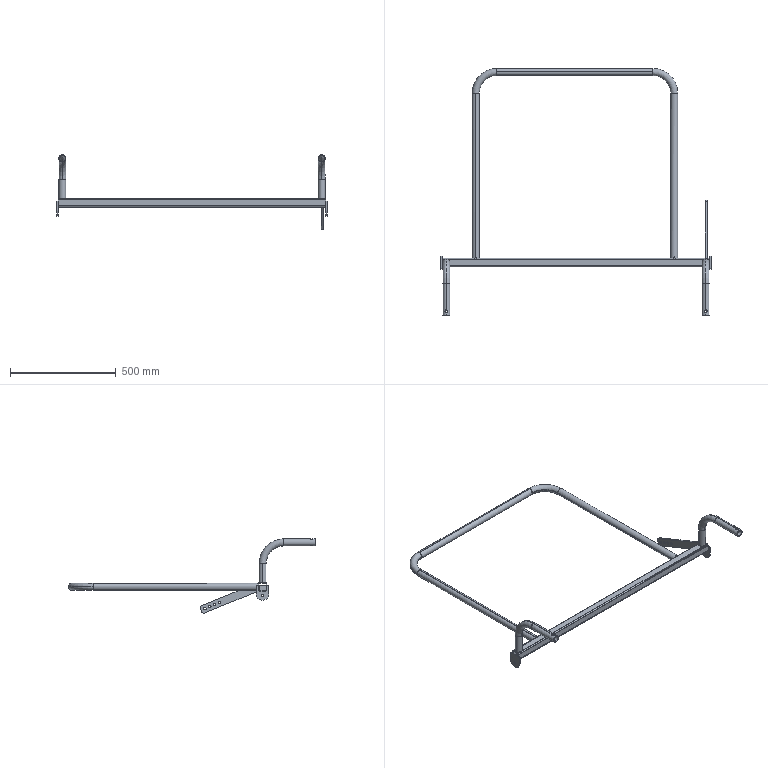Part | SolidWorks | features ICE 4, Fillet 2, WeldCornerFeat 2, WeldMemberFeat 2, 3DProfileFeature 1, MirrorSolid 1, WeldmentFeature 1 | 15 solids | 139 faces | box 1275 x 1167 x 350.869 mm | volume 1494130 mm3 | cylinder 65 | plane 58 | torus 16 | commonest cylinder face diameters 12 x16 28.3 x14 33.3 x14 13 x8 6 x4 10 x4